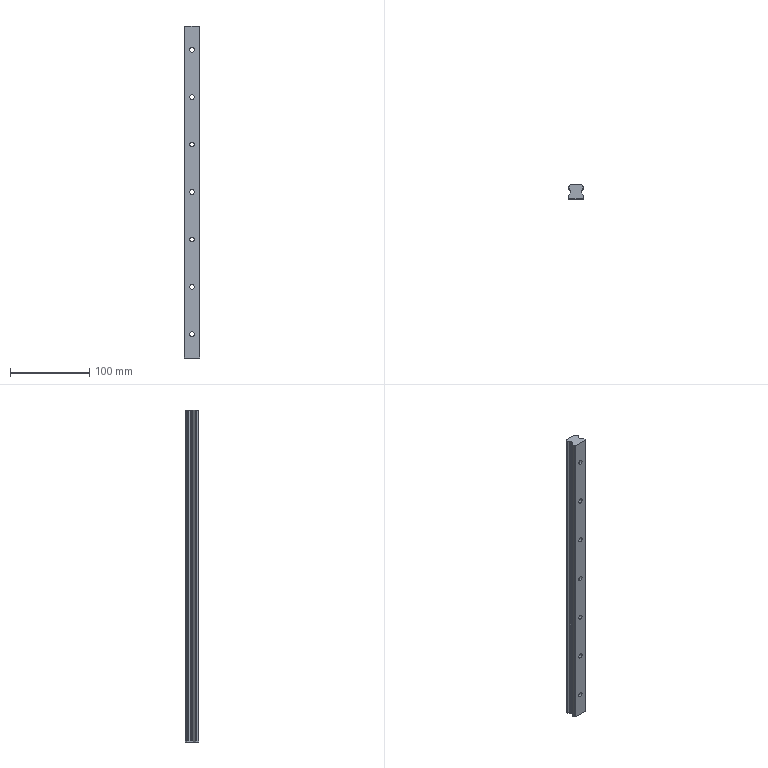Part | SolidWorks | features BaseBody 1 | 1 solid | 79 faces | box 20 x 17.5 x 420 mm | volume 119541 mm3 | cylinder 50 | plane 29 | commonest cylinder face diameters 6 x14 9.5 x14 1 x12 2 x6 4.06 x4